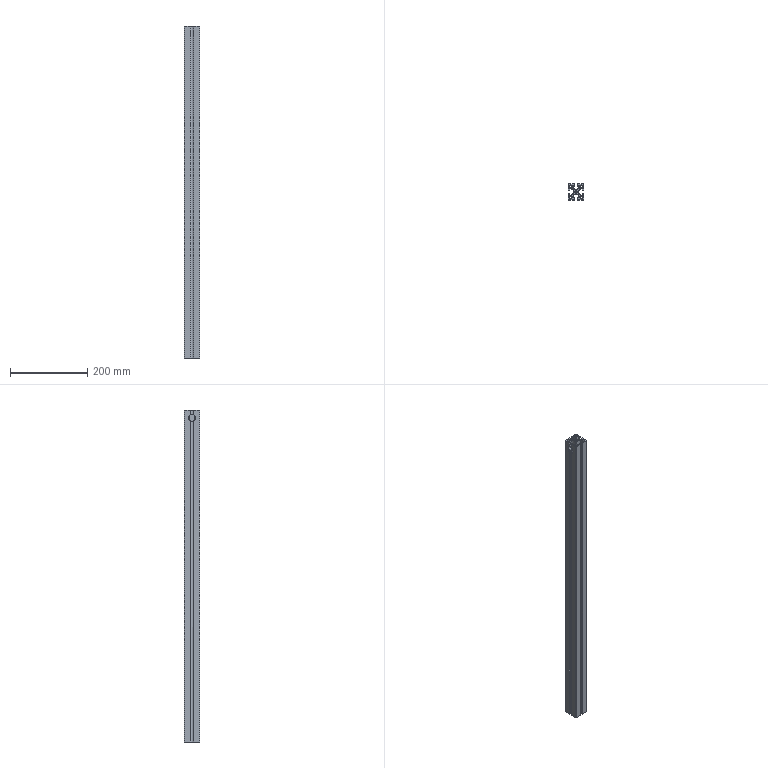Part | STEP file | 09-05 aluminium profile 4040-860 | 1 solid | 74 faces | box 40 x 40 x 860 mm | volume 605454 mm3 | plane 48 | cylinder 26 | commonest cylinder face diameters 8 x8 19 x8 2 x4 18.5 x4 6.8 x2